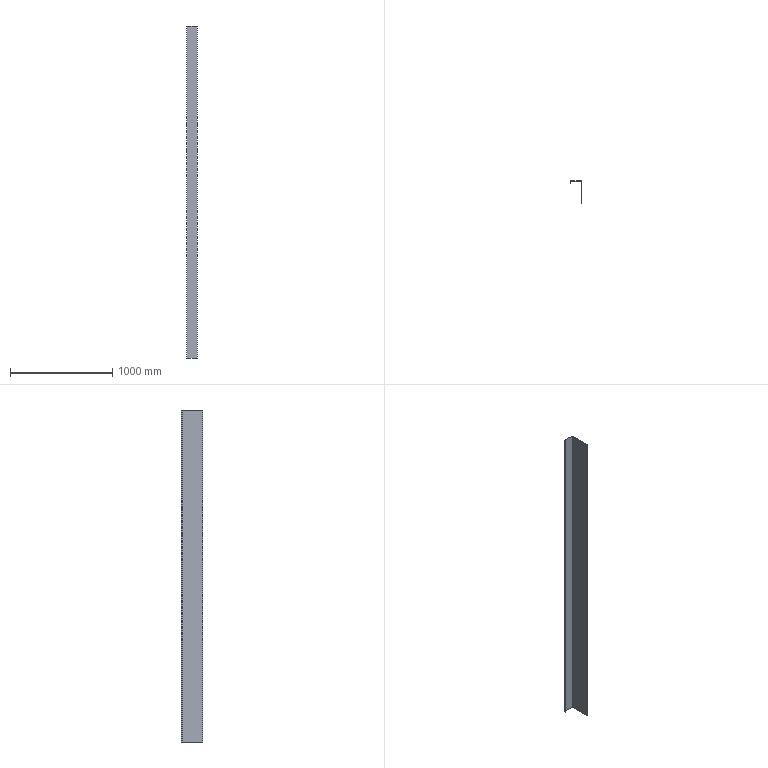Part | NX | features BREP 1 | 1 solid | 10 faces | box 103 x 211.5 x 3250 mm | volume 1599000 mm3 | plane 10
STEP:
#1=CARTESIAN_POINT('',(1.5,211.5,3250.));
#2=VERTEX_POINT('',#1);
#3=CARTESIAN_POINT('',(1.5,211.5,0.));
#4=VERTEX_POINT('',#3);
#5=CARTESIAN_POINT('',(1.5,211.5,3250.));
#6=DIRECTION('',(0.,0.,-1.));
#7=VECTOR('',#6,1000.);
#8=LINE('',#5,#7);
#9=EDGE_CURVE('',#2,#4,#8,.T.);
#10=ORIENTED_EDGE('',*,*,#9,.F.);
#11=CARTESIAN_POINT('',(1.5,0.,3250.));
#12=VERTEX_POINT('',#11);
#13=CARTESIAN_POINT('',(1.5,0.,3250.));
#14=DIRECTION('',(0.,1.,0.));
#15=VECTOR('',#14,1000.);
#16=LINE('',#13,#15);
#17=EDGE_CURVE('',#12,#2,#16,.T.);
#18=ORIENTED_EDGE('',*,*,#17,.F.);
#19=CARTESIAN_POINT('',(1.5,0.,0.));
#20=VERTEX_POINT('',#19);
#21=CARTESIAN_POINT('',(1.5,0.,3250.));
#22=DIRECTION('',(0.,0.,1.));
#23=VECTOR('',#22,1000.);
#24=LINE('',#21,#23);
#25=EDGE_CURVE('',#20,#12,#24,.T.);
#26=ORIENTED_EDGE('',*,*,#25,.F.);
#27=CARTESIAN_POINT('',(1.5,0.,0.));
#28=DIRECTION('',(0.,-1.,0.));
#29=VECTOR('',#28,1000.);
#30=LINE('',#27,#29);
#31=EDGE_CURVE('',#4,#20,#30,.T.);
#32=ORIENTED_EDGE('',*,*,#31,.F.);
#33=EDGE_LOOP('',(#10,#18,#26,#32));
#34=FACE_BOUND('',#33,.T.);
#35=CARTESIAN_POINT('',(1.5,0.,3250.));
#36=DIRECTION('',(-1.,0.,0.));
#37=DIRECTION('',(0.,0.,1.));
#38=AXIS2_PLACEMENT_3D('',#35,#36,#37);
#39=PLANE('',#38);
#40=ADVANCED_FACE('',(#34),#39,.F.);
#41=CARTESIAN_POINT('',(0.,210.,0.));
#42=VERTEX_POINT('',#41);
#43=CARTESIAN_POINT('',(0.,0.,0.));
#44=VERTEX_POINT('',#43);
#45=CARTESIAN_POINT('',(0.,0.,0.));
#46=DIRECTION('',(0.,-1.,0.));
#47=VECTOR('',#46,1000.);
#48=LINE('',#45,#47);
#49=EDGE_CURVE('',#42,#44,#48,.T.);
#50=ORIENTED_EDGE('',*,*,#49,.F.);
#51=CARTESIAN_POINT('',(-100.,210.,0.));
#52=VERTEX_POINT('',#51);
#53=CARTESIAN_POINT('',(1.5,210.,0.));
#54=DIRECTION('',(1.,0.,0.));
#55=VECTOR('',#54,1000.);
#56=LINE('',#53,#55);
#57=EDGE_CURVE('',#52,#42,#56,.T.);
#58=ORIENTED_EDGE('',*,*,#57,.F.);
#59=CARTESIAN_POINT('',(-100.,195.,0.));
#60=VERTEX_POINT('',#59);
#61=CARTESIAN_POINT('',(-100.,0.,0.));
#62=DIRECTION('',(0.,1.,0.));
#63=VECTOR('',#62,1000.);
#64=LINE('',#61,#63);
#65=EDGE_CURVE('',#60,#52,#64,.T.);
#66=ORIENTED_EDGE('',*,*,#65,.F.);
#67=CARTESIAN_POINT('',(-101.5,195.,0.));
#68=VERTEX_POINT('',#67);
#69=CARTESIAN_POINT('',(-101.5,195.,0.));
#70=DIRECTION('',(-1.,0.,0.));
#71=VECTOR('',#70,1000.);
#72=LINE('',#69,#71);
#73=EDGE_CURVE('',#60,#68,#72,.T.);
#74=ORIENTED_EDGE('',*,*,#73,.T.);
#75=CARTESIAN_POINT('',(-101.5,211.5,0.));
#76=VERTEX_POINT('',#75);
#77=CARTESIAN_POINT('',(-101.5,0.,0.));
#78=DIRECTION('',(0.,-1.,0.));
#79=VECTOR('',#78,1000.);
#80=LINE('',#77,#79);
#81=EDGE_CURVE('',#76,#68,#80,.T.);
#82=ORIENTED_EDGE('',*,*,#81,.F.);
#83=CARTESIAN_POINT('',(1.5,211.5,0.));
#84=DIRECTION('',(-1.,0.,0.));
#85=VECTOR('',#84,1000.);
#86=LINE('',#83,#85);
#87=EDGE_CURVE('',#4,#76,#86,.T.);
#88=ORIENTED_EDGE('',*,*,#87,.F.);
#89=ORIENTED_EDGE('',*,*,#31,.T.);
#90=CARTESIAN_POINT('',(1.5,0.,0.));
#91=DIRECTION('',(1.,0.,0.));
#92=VECTOR('',#91,1000.);
#93=LINE('',#90,#92);
#94=EDGE_CURVE('',#44,#20,#93,.T.);
#95=ORIENTED_EDGE('',*,*,#94,.F.);
#96=EDGE_LOOP('',(#50,#58,#66,#74,#82,#88,#89,#95));
#97=FACE_BOUND('',#96,.T.);
#98=CARTESIAN_POINT('',(1.5,0.,0.));
#99=DIRECTION('',(0.,0.,1.));
#100=DIRECTION('',(1.,0.,0.));
#101=AXIS2_PLACEMENT_3D('',#98,#99,#100);
#102=PLANE('',#101);
#103=ADVANCED_FACE('',(#97),#102,.F.);
#104=CARTESIAN_POINT('',(-101.5,211.5,3250.));
#105=VERTEX_POINT('',#104);
#106=CARTESIAN_POINT('',(-101.5,211.5,3250.));
#107=DIRECTION('',(0.,0.,-1.));
#108=VECTOR('',#107,1000.);
#109=LINE('',#106,#108);
#110=EDGE_CURVE('',#105,#76,#109,.T.);
#111=ORIENTED_EDGE('',*,*,#110,.F.);
#112=CARTESIAN_POINT('',(1.5,211.5,3250.));
#113=DIRECTION('',(-1.,0.,0.));
#114=VECTOR('',#113,1000.);
#115=LINE('',#112,#114);
#116=EDGE_CURVE('',#2,#105,#115,.T.);
#117=ORIENTED_EDGE('',*,*,#116,.F.);
#118=ORIENTED_EDGE('',*,*,#9,.T.);
#119=ORIENTED_EDGE('',*,*,#87,.T.);
#120=EDGE_LOOP('',(#111,#117,#118,#119));
#121=FACE_BOUND('',#120,.T.);
#122=CARTESIAN_POINT('',(1.5,211.5,3250.));
#123=DIRECTION('',(0.,-1.,0.));
#124=DIRECTION('',(0.,0.,-1.));
#125=AXIS2_PLACEMENT_3D('',#122,#123,#124);
#126=PLANE('',#125);
#127=ADVANCED_FACE('',(#121),#126,.F.);
#128=CARTESIAN_POINT('',(-100.,210.,3250.));
#129=VERTEX_POINT('',#128);
#130=CARTESIAN_POINT('',(0.,210.,3250.));
#131=VERTEX_POINT('',#130);
#132=CARTESIAN_POINT('',(1.5,210.,3250.));
#133=DIRECTION('',(1.,0.,0.));
#134=VECTOR('',#133,1000.);
#135=LINE('',#132,#134);
#136=EDGE_CURVE('',#129,#131,#135,.T.);
#137=ORIENTED_EDGE('',*,*,#136,.T.);
#138=CARTESIAN_POINT('',(0.,0.,3250.));
#139=VERTEX_POINT('',#138);
#140=CARTESIAN_POINT('',(0.,0.,3250.));
#141=DIRECTION('',(0.,-1.,0.));
#142=VECTOR('',#141,1000.);
#143=LINE('',#140,#142);
#144=EDGE_CURVE('',#131,#139,#143,.T.);
#145=ORIENTED_EDGE('',*,*,#144,.T.);
#146=CARTESIAN_POINT('',(1.5,0.,3250.));
#147=DIRECTION('',(1.,0.,0.));
#148=VECTOR('',#147,1000.);
#149=LINE('',#146,#148);
#150=EDGE_CURVE('',#139,#12,#149,.T.);
#151=ORIENTED_EDGE('',*,*,#150,.T.);
#152=ORIENTED_EDGE('',*,*,#17,.T.);
#153=ORIENTED_EDGE('',*,*,#116,.T.);
#154=CARTESIAN_POINT('',(-101.5,195.,3250.));
#155=VERTEX_POINT('',#154);
#156=CARTESIAN_POINT('',(-101.5,0.,3250.));
#157=DIRECTION('',(0.,-1.,0.));
#158=VECTOR('',#157,1000.);
#159=LINE('',#156,#158);
#160=EDGE_CURVE('',#105,#155,#159,.T.);
#161=ORIENTED_EDGE('',*,*,#160,.T.);
#162=CARTESIAN_POINT('',(-100.,195.,3250.));
#163=VERTEX_POINT('',#162);
#164=CARTESIAN_POINT('',(-101.5,195.,3250.));
#165=DIRECTION('',(1.,0.,0.));
#166=VECTOR('',#165,1000.);
#167=LINE('',#164,#166);
#168=EDGE_CURVE('',#155,#163,#167,.T.);
#169=ORIENTED_EDGE('',*,*,#168,.T.);
#170=CARTESIAN_POINT('',(-100.,0.,3250.));
#171=DIRECTION('',(0.,1.,0.));
#172=VECTOR('',#171,1000.);
#173=LINE('',#170,#172);
#174=EDGE_CURVE('',#163,#129,#173,.T.);
#175=ORIENTED_EDGE('',*,*,#174,.T.);
#176=EDGE_LOOP('',(#137,#145,#151,#152,#153,#161,#169,#175));
#177=FACE_BOUND('',#176,.T.);
#178=CARTESIAN_POINT('',(1.5,0.,3250.));
#179=DIRECTION('',(0.,0.,1.));
#180=DIRECTION('',(1.,0.,0.));
#181=AXIS2_PLACEMENT_3D('',#178,#179,#180);
#182=PLANE('',#181);
#183=ADVANCED_FACE('',(#177),#182,.T.);
#184=ORIENTED_EDGE('',*,*,#25,.T.);
#185=ORIENTED_EDGE('',*,*,#150,.F.);
#186=CARTESIAN_POINT('',(0.,0.,3250.));
#187=DIRECTION('',(0.,0.,1.));
#188=VECTOR('',#187,1000.);
#189=LINE('',#186,#188);
#190=EDGE_CURVE('',#44,#139,#189,.T.);
#191=ORIENTED_EDGE('',*,*,#190,.F.);
#192=ORIENTED_EDGE('',*,*,#94,.T.);
#193=EDGE_LOOP('',(#184,#185,#191,#192));
#194=FACE_BOUND('',#193,.T.);
#195=CARTESIAN_POINT('',(0.,0.,3250.));
#196=DIRECTION('',(0.,1.,0.));
#197=DIRECTION('',(1.,0.,0.));
#198=AXIS2_PLACEMENT_3D('',#195,#196,#197);
#199=PLANE('',#198);
#200=ADVANCED_FACE('',(#194),#199,.F.);
#201=ORIENTED_EDGE('',*,*,#190,.T.);
#202=ORIENTED_EDGE('',*,*,#144,.F.);
#203=CARTESIAN_POINT('',(0.,210.,3250.));
#204=DIRECTION('',(0.,0.,1.));
#205=VECTOR('',#204,1000.);
#206=LINE('',#203,#205);
#207=EDGE_CURVE('',#42,#131,#206,.T.);
#208=ORIENTED_EDGE('',*,*,#207,.F.);
#209=ORIENTED_EDGE('',*,*,#49,.T.);
#210=EDGE_LOOP('',(#201,#202,#208,#209));
#211=FACE_BOUND('',#210,.T.);
#212=CARTESIAN_POINT('',(0.,0.,3250.));
#213=DIRECTION('',(1.,0.,0.));
#214=DIRECTION('',(0.,1.,0.));
#215=AXIS2_PLACEMENT_3D('',#212,#213,#214);
#216=PLANE('',#215);
#217=ADVANCED_FACE('',(#211),#216,.F.);
#218=ORIENTED_EDGE('',*,*,#207,.T.);
#219=ORIENTED_EDGE('',*,*,#136,.F.);
#220=CARTESIAN_POINT('',(-100.,210.,3250.));
#221=DIRECTION('',(0.,0.,1.));
#222=VECTOR('',#221,1000.);
#223=LINE('',#220,#222);
#224=EDGE_CURVE('',#52,#129,#223,.T.);
#225=ORIENTED_EDGE('',*,*,#224,.F.);
#226=ORIENTED_EDGE('',*,*,#57,.T.);
#227=EDGE_LOOP('',(#218,#219,#225,#226));
#228=FACE_BOUND('',#227,.T.);
#229=CARTESIAN_POINT('',(0.,210.,3250.));
#230=DIRECTION('',(0.,1.,0.));
#231=DIRECTION('',(1.,0.,0.));
#232=AXIS2_PLACEMENT_3D('',#229,#230,#231);
#233=PLANE('',#232);
#234=ADVANCED_FACE('',(#228),#233,.F.);
#235=ORIENTED_EDGE('',*,*,#224,.T.);
#236=ORIENTED_EDGE('',*,*,#174,.F.);
#237=CARTESIAN_POINT('',(-100.,195.,3250.));
#238=DIRECTION('',(0.,0.,1.));
#239=VECTOR('',#238,1000.);
#240=LINE('',#237,#239);
#241=EDGE_CURVE('',#60,#163,#240,.T.);
#242=ORIENTED_EDGE('',*,*,#241,.F.);
#243=ORIENTED_EDGE('',*,*,#65,.T.);
#244=EDGE_LOOP('',(#235,#236,#242,#243));
#245=FACE_BOUND('',#244,.T.);
#246=CARTESIAN_POINT('',(-100.,210.,3250.));
#247=DIRECTION('',(-1.,0.,0.));
#248=DIRECTION('',(0.,0.,1.));
#249=AXIS2_PLACEMENT_3D('',#246,#247,#248);
#250=PLANE('',#249);
#251=ADVANCED_FACE('',(#245),#250,.F.);
#252=CARTESIAN_POINT('',(-101.5,195.,3250.));
#253=DIRECTION('',(0.,0.,-1.));
#254=VECTOR('',#253,1000.);
#255=LINE('',#252,#254);
#256=EDGE_CURVE('',#155,#68,#255,.T.);
#257=ORIENTED_EDGE('',*,*,#256,.F.);
#258=ORIENTED_EDGE('',*,*,#160,.F.);
#259=ORIENTED_EDGE('',*,*,#110,.T.);
#260=ORIENTED_EDGE('',*,*,#81,.T.);
#261=EDGE_LOOP('',(#257,#258,#259,#260));
#262=FACE_BOUND('',#261,.T.);
#263=CARTESIAN_POINT('',(-101.5,211.5,3250.));
#264=DIRECTION('',(1.,0.,0.));
#265=DIRECTION('',(0.,1.,0.));
#266=AXIS2_PLACEMENT_3D('',#263,#264,#265);
#267=PLANE('',#266);
#268=ADVANCED_FACE('',(#262),#267,.F.);
#269=ORIENTED_EDGE('',*,*,#241,.T.);
#270=ORIENTED_EDGE('',*,*,#168,.F.);
#271=ORIENTED_EDGE('',*,*,#256,.T.);
#272=ORIENTED_EDGE('',*,*,#73,.F.);
#273=EDGE_LOOP('',(#269,#270,#271,#272));
#274=FACE_BOUND('',#273,.T.);
#275=CARTESIAN_POINT('',(-101.5,195.,3250.));
#276=DIRECTION('',(0.,1.,0.));
#277=DIRECTION('',(1.,0.,0.));
#278=AXIS2_PLACEMENT_3D('',#275,#276,#277);
#279=PLANE('',#278);
#280=ADVANCED_FACE('',(#274),#279,.F.);
#281=CLOSED_SHELL('',(#40,#103,#127,#183,#200,#217,#234,#251,#268,#280));
#282=MANIFOLD_SOLID_BREP('',#281);
#283=(LENGTH_UNIT()NAMED_UNIT(*)SI_UNIT(.MILLI.,.METRE.));
#284=UNCERTAINTY_MEASURE_WITH_UNIT(LENGTH_MEASURE(0.00001),#283,'','');
#285=(NAMED_UNIT(*)PLANE_ANGLE_UNIT()SI_UNIT($,.RADIAN.));
#286=(NAMED_UNIT(*)SI_UNIT($,.STERADIAN.)SOLID_ANGLE_UNIT());
#287=(GEOMETRIC_REPRESENTATION_CONTEXT(3)GLOBAL_UNCERTAINTY_ASSIGNED_CONTEXT((#284))GLOBAL_UNIT_ASSIGNED_CONTEXT((#283,#285,#286))REPRESENTATION_CONTEXT('',''));
#288=ADVANCED_BREP_SHAPE_REPRESENTATION('',(#282),#287);